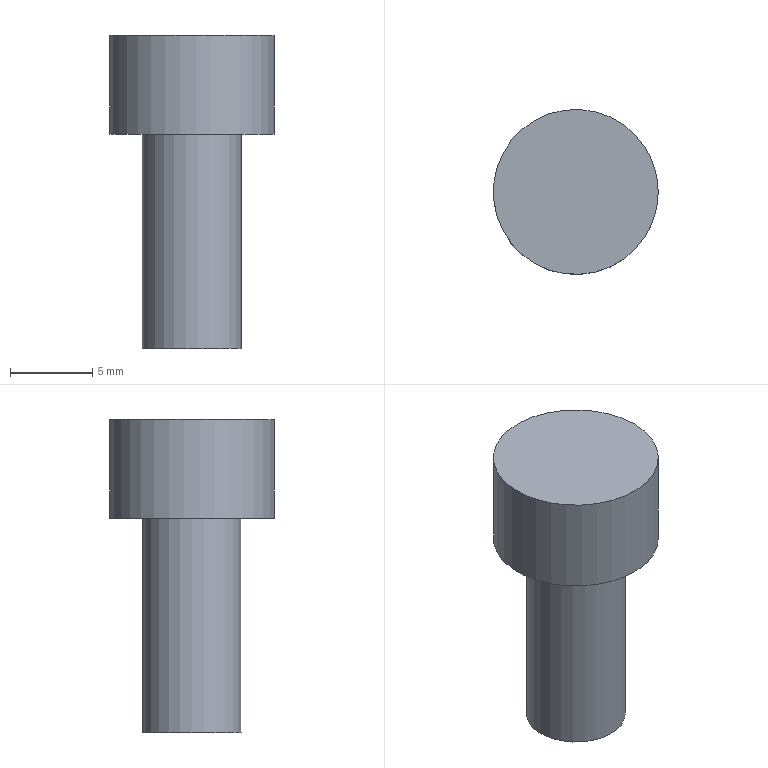Part | NX | features DATUM_CSYS 2, EXTRUDE 2, SKETCH 1 | 1 solid | 5 faces | box 10 x 10 x 19 mm | volume 838.805 mm3 | plane 3 | cylinder 2 | commonest cylinder face diameters 6 x1 10 x1
STEP:
#1=CARTESIAN_POINT('',(5.,0.,6.));
#2=VERTEX_POINT('',#1);
#3=CARTESIAN_POINT('',(0.,0.,6.));
#4=DIRECTION('',(0.,0.,1.));
#5=DIRECTION('',(1.,0.,0.));
#6=AXIS2_PLACEMENT_3D('',#3,#4,#5);
#7=CIRCLE('',#6,5.);
#8=EDGE_CURVE('',#2,#2,#7,.T.);
#9=ORIENTED_EDGE('',*,*,#8,.F.);
#10=EDGE_LOOP('',(#9));
#11=FACE_BOUND('',#10,.T.);
#12=CARTESIAN_POINT('',(5.,0.,0.));
#13=VERTEX_POINT('',#12);
#14=CARTESIAN_POINT('',(0.,0.,0.));
#15=DIRECTION('',(0.,0.,1.));
#16=DIRECTION('',(1.,0.,0.));
#17=AXIS2_PLACEMENT_3D('',#14,#15,#16);
#18=CIRCLE('',#17,5.);
#19=EDGE_CURVE('',#13,#13,#18,.T.);
#20=ORIENTED_EDGE('',*,*,#19,.T.);
#21=EDGE_LOOP('',(#20));
#22=FACE_BOUND('',#21,.T.);
#23=CARTESIAN_POINT('',(0.,0.,6.));
#24=DIRECTION('',(0.,0.,-1.));
#25=DIRECTION('',(-1.,0.,0.));
#26=AXIS2_PLACEMENT_3D('',#23,#24,#25);
#27=CYLINDRICAL_SURFACE('',#26,5.);
#28=ADVANCED_FACE('',(#11,#22),#27,.T.);
#29=ORIENTED_EDGE('',*,*,#8,.T.);
#30=EDGE_LOOP('',(#29));
#31=FACE_BOUND('',#30,.T.);
#32=CARTESIAN_POINT('',(0.,0.,6.));
#33=DIRECTION('',(0.,0.,1.));
#34=DIRECTION('',(1.,0.,0.));
#35=AXIS2_PLACEMENT_3D('',#32,#33,#34);
#36=PLANE('',#35);
#37=ADVANCED_FACE('',(#31),#36,.T.);
#38=CARTESIAN_POINT('',(3.,0.,0.));
#39=VERTEX_POINT('',#38);
#40=CARTESIAN_POINT('',(0.,0.,0.));
#41=DIRECTION('',(0.,0.,-1.));
#42=DIRECTION('',(1.,0.,0.));
#43=AXIS2_PLACEMENT_3D('',#40,#41,#42);
#44=CIRCLE('',#43,3.);
#45=EDGE_CURVE('',#39,#39,#44,.T.);
#46=ORIENTED_EDGE('',*,*,#45,.F.);
#47=EDGE_LOOP('',(#46));
#48=FACE_BOUND('',#47,.T.);
#49=ORIENTED_EDGE('',*,*,#19,.F.);
#50=EDGE_LOOP('',(#49));
#51=FACE_BOUND('',#50,.T.);
#52=CARTESIAN_POINT('',(0.,0.,0.));
#53=DIRECTION('',(0.,0.,1.));
#54=DIRECTION('',(1.,0.,0.));
#55=AXIS2_PLACEMENT_3D('',#52,#53,#54);
#56=PLANE('',#55);
#57=ADVANCED_FACE('',(#48,#51),#56,.F.);
#58=CARTESIAN_POINT('',(3.,0.,-13.));
#59=VERTEX_POINT('',#58);
#60=CARTESIAN_POINT('',(0.,0.,-13.));
#61=DIRECTION('',(0.,0.,-1.));
#62=DIRECTION('',(1.,0.,0.));
#63=AXIS2_PLACEMENT_3D('',#60,#61,#62);
#64=CIRCLE('',#63,3.);
#65=EDGE_CURVE('',#59,#59,#64,.T.);
#66=ORIENTED_EDGE('',*,*,#65,.F.);
#67=EDGE_LOOP('',(#66));
#68=FACE_BOUND('',#67,.T.);
#69=ORIENTED_EDGE('',*,*,#45,.T.);
#70=EDGE_LOOP('',(#69));
#71=FACE_BOUND('',#70,.T.);
#72=CARTESIAN_POINT('',(0.,0.,-13.));
#73=DIRECTION('',(0.,0.,1.));
#74=DIRECTION('',(1.,0.,0.));
#75=AXIS2_PLACEMENT_3D('',#72,#73,#74);
#76=CYLINDRICAL_SURFACE('',#75,3.);
#77=ADVANCED_FACE('',(#68,#71),#76,.T.);
#78=ORIENTED_EDGE('',*,*,#65,.T.);
#79=EDGE_LOOP('',(#78));
#80=FACE_BOUND('',#79,.T.);
#81=CARTESIAN_POINT('',(0.,0.,-13.));
#82=DIRECTION('',(0.,0.,-1.));
#83=DIRECTION('',(-1.,0.,0.));
#84=AXIS2_PLACEMENT_3D('',#81,#82,#83);
#85=PLANE('',#84);
#86=ADVANCED_FACE('',(#80),#85,.T.);
#87=CLOSED_SHELL('',(#28,#37,#57,#77,#86));
#88=MANIFOLD_SOLID_BREP('',#87);
#89=(LENGTH_UNIT()NAMED_UNIT(*)SI_UNIT(.MILLI.,.METRE.));
#90=UNCERTAINTY_MEASURE_WITH_UNIT(LENGTH_MEASURE(0.00001),#89,'','');
#91=(NAMED_UNIT(*)PLANE_ANGLE_UNIT()SI_UNIT($,.RADIAN.));
#92=(NAMED_UNIT(*)SI_UNIT($,.STERADIAN.)SOLID_ANGLE_UNIT());
#93=(GEOMETRIC_REPRESENTATION_CONTEXT(3)GLOBAL_UNCERTAINTY_ASSIGNED_CONTEXT((#90))GLOBAL_UNIT_ASSIGNED_CONTEXT((#89,#91,#92))REPRESENTATION_CONTEXT('',''));
#94=ADVANCED_BREP_SHAPE_REPRESENTATION('',(#88),#93);